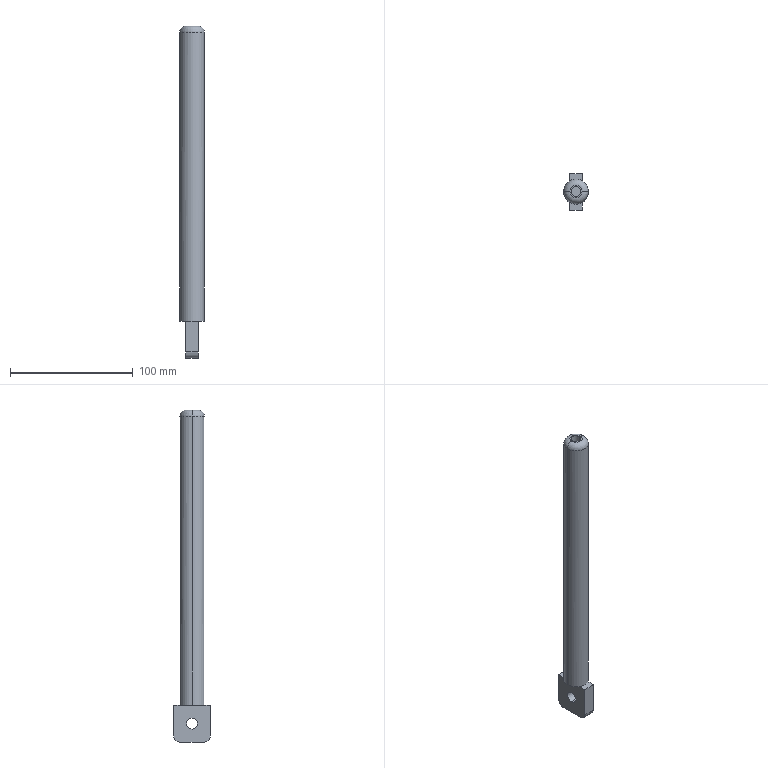Part | SolidWorks | features ICE 3, Fillet 2, Extrusion 1 | 1 solid | 21 faces | box 20 x 30 x 270 mm | volume 82350 mm3 | plane 11 | cylinder 8 | torus 2 | commonest cylinder face diameters 8 x2 9 x2 10 x2 20 x2
STEP:
#1=CARTESIAN_POINT('',(-4.,0.,220.));
#2=VERTEX_POINT('',#1);
#3=CARTESIAN_POINT('',(4.,0.,220.));
#4=VERTEX_POINT('',#3);
#5=CARTESIAN_POINT('',(0.,0.,220.));
#6=DIRECTION('',(0.,0.,1.));
#7=DIRECTION('',(1.,0.,0.));
#8=AXIS2_PLACEMENT_3D('',#5,#6,#7);
#9=CIRCLE('',#8,4.);
#10=EDGE_CURVE('',#2,#4,#9,.T.);
#11=ORIENTED_EDGE('',*,*,#10,.F.);
#12=CARTESIAN_POINT('',(-4.,0.,240.));
#13=VERTEX_POINT('',#12);
#14=CARTESIAN_POINT('',(-4.,0.,220.));
#15=DIRECTION('',(0.,0.,1.));
#16=VECTOR('',#15,1000.);
#17=LINE('',#14,#16);
#18=EDGE_CURVE('',#2,#13,#17,.T.);
#19=ORIENTED_EDGE('',*,*,#18,.T.);
#20=CARTESIAN_POINT('',(4.,0.,240.));
#21=VERTEX_POINT('',#20);
#22=CARTESIAN_POINT('',(0.,0.,240.));
#23=DIRECTION('',(0.,0.,1.));
#24=DIRECTION('',(1.,0.,0.));
#25=AXIS2_PLACEMENT_3D('',#22,#23,#24);
#26=CIRCLE('',#25,4.);
#27=EDGE_CURVE('',#13,#21,#26,.T.);
#28=ORIENTED_EDGE('',*,*,#27,.T.);
#29=CARTESIAN_POINT('',(4.,0.,220.));
#30=DIRECTION('',(0.,0.,1.));
#31=VECTOR('',#30,1000.);
#32=LINE('',#29,#31);
#33=EDGE_CURVE('',#4,#21,#32,.T.);
#34=ORIENTED_EDGE('',*,*,#33,.F.);
#35=EDGE_LOOP('',(#11,#19,#28,#34));
#36=FACE_OUTER_BOUND('',#35,.T.);
#37=CARTESIAN_POINT('',(0.,0.,220.));
#38=DIRECTION('',(0.,0.,1.));
#39=DIRECTION('',(1.,0.,0.));
#40=AXIS2_PLACEMENT_3D('',#37,#38,#39);
#41=CYLINDRICAL_SURFACE('',#40,4.);
#42=ADVANCED_FACE('',(#36),#41,.F.);
#43=CARTESIAN_POINT('',(-10.,0.,235.));
#44=VERTEX_POINT('',#43);
#45=CARTESIAN_POINT('',(10.,0.,235.));
#46=VERTEX_POINT('',#45);
#47=CARTESIAN_POINT('',(0.,0.,235.));
#48=DIRECTION('',(0.,0.,-1.));
#49=DIRECTION('',(1.,0.,0.));
#50=AXIS2_PLACEMENT_3D('',#47,#48,#49);
#51=CIRCLE('',#50,10.);
#52=EDGE_CURVE('',#44,#46,#51,.T.);
#53=ORIENTED_EDGE('',*,*,#52,.F.);
#54=CARTESIAN_POINT('',(-5.,0.,240.));
#55=VERTEX_POINT('',#54);
#56=CARTESIAN_POINT('',(-5.,0.,235.));
#57=DIRECTION('',(0.,1.,0.));
#58=DIRECTION('',(-1.,0.,0.));
#59=AXIS2_PLACEMENT_3D('',#56,#57,#58);
#60=CIRCLE('',#59,5.);
#61=EDGE_CURVE('',#44,#55,#60,.T.);
#62=ORIENTED_EDGE('',*,*,#61,.T.);
#63=CARTESIAN_POINT('',(5.,0.,240.));
#64=VERTEX_POINT('',#63);
#65=CARTESIAN_POINT('',(0.,0.,240.));
#66=DIRECTION('',(0.,0.,1.));
#67=DIRECTION('',(1.,0.,0.));
#68=AXIS2_PLACEMENT_3D('',#65,#66,#67);
#69=CIRCLE('',#68,5.);
#70=EDGE_CURVE('',#64,#55,#69,.T.);
#71=ORIENTED_EDGE('',*,*,#70,.F.);
#72=CARTESIAN_POINT('',(5.,0.,235.));
#73=DIRECTION('',(0.,-1.,0.));
#74=DIRECTION('',(0.,0.,-1.));
#75=AXIS2_PLACEMENT_3D('',#72,#73,#74);
#76=CIRCLE('',#75,5.);
#77=EDGE_CURVE('',#46,#64,#76,.T.);
#78=ORIENTED_EDGE('',*,*,#77,.F.);
#79=EDGE_LOOP('',(#53,#62,#71,#78));
#80=FACE_OUTER_BOUND('',#79,.T.);
#81=CARTESIAN_POINT('',(0.,0.,235.));
#82=DIRECTION('',(0.,0.,1.));
#83=DIRECTION('',(1.,0.,0.));
#84=AXIS2_PLACEMENT_3D('',#81,#82,#83);
#85=TOROIDAL_SURFACE('',#84,5.,5.);
#86=ADVANCED_FACE('',(#80),#85,.T.);
#87=CARTESIAN_POINT('',(-5.,0.,-19.5));
#88=VERTEX_POINT('',#87);
#89=CARTESIAN_POINT('',(-5.,0.,-10.5));
#90=VERTEX_POINT('',#89);
#91=CARTESIAN_POINT('',(-5.,0.,-15.));
#92=DIRECTION('',(-1.,0.,0.));
#93=DIRECTION('',(0.,0.,1.));
#94=AXIS2_PLACEMENT_3D('',#91,#92,#93);
#95=CIRCLE('',#94,4.5);
#96=EDGE_CURVE('',#88,#90,#95,.T.);
#97=ORIENTED_EDGE('',*,*,#96,.T.);
#98=CARTESIAN_POINT('',(5.,0.,-10.5));
#99=VERTEX_POINT('',#98);
#100=CARTESIAN_POINT('',(-33.,0.,-10.5));
#101=DIRECTION('',(1.,0.,0.));
#102=VECTOR('',#101,1000.);
#103=LINE('',#100,#102);
#104=EDGE_CURVE('',#90,#99,#103,.T.);
#105=ORIENTED_EDGE('',*,*,#104,.T.);
#106=CARTESIAN_POINT('',(5.,0.,-19.5));
#107=VERTEX_POINT('',#106);
#108=CARTESIAN_POINT('',(5.,0.,-15.));
#109=DIRECTION('',(1.,0.,0.));
#110=DIRECTION('',(0.,0.,-1.));
#111=AXIS2_PLACEMENT_3D('',#108,#109,#110);
#112=CIRCLE('',#111,4.5);
#113=EDGE_CURVE('',#99,#107,#112,.T.);
#114=ORIENTED_EDGE('',*,*,#113,.T.);
#115=CARTESIAN_POINT('',(-33.,0.,-19.5));
#116=DIRECTION('',(1.,0.,0.));
#117=VECTOR('',#116,1000.);
#118=LINE('',#115,#117);
#119=EDGE_CURVE('',#88,#107,#118,.T.);
#120=ORIENTED_EDGE('',*,*,#119,.F.);
#121=EDGE_LOOP('',(#97,#105,#114,#120));
#122=FACE_OUTER_BOUND('',#121,.T.);
#123=CARTESIAN_POINT('',(-33.,0.,-15.));
#124=DIRECTION('',(1.,0.,0.));
#125=DIRECTION('',(0.,0.,-1.));
#126=AXIS2_PLACEMENT_3D('',#123,#124,#125);
#127=CYLINDRICAL_SURFACE('',#126,4.5);
#128=ADVANCED_FACE('',(#122),#127,.F.);
#129=ORIENTED_EDGE('',*,*,#52,.T.);
#130=CARTESIAN_POINT('',(10.,0.,0.));
#131=VERTEX_POINT('',#130);
#132=CARTESIAN_POINT('',(10.,0.,240.));
#133=DIRECTION('',(0.,0.,-1.));
#134=VECTOR('',#133,1000.);
#135=LINE('',#132,#134);
#136=EDGE_CURVE('',#46,#131,#135,.T.);
#137=ORIENTED_EDGE('',*,*,#136,.T.);
#138=CARTESIAN_POINT('',(5.,8.66,0.));
#139=VERTEX_POINT('',#138);
#140=CARTESIAN_POINT('',(0.,0.,0.));
#141=DIRECTION('',(0.,0.,1.));
#142=DIRECTION('',(1.,0.,0.));
#143=AXIS2_PLACEMENT_3D('',#140,#141,#142);
#144=CIRCLE('',#143,10.);
#145=EDGE_CURVE('',#131,#139,#144,.T.);
#146=ORIENTED_EDGE('',*,*,#145,.T.);
#147=CARTESIAN_POINT('',(-5.,8.66,0.));
#148=VERTEX_POINT('',#147);
#149=CARTESIAN_POINT('',(0.,0.,0.));
#150=DIRECTION('',(0.,0.,1.));
#151=DIRECTION('',(1.,0.,0.));
#152=AXIS2_PLACEMENT_3D('',#149,#150,#151);
#153=CIRCLE('',#152,10.);
#154=EDGE_CURVE('',#139,#148,#153,.T.);
#155=ORIENTED_EDGE('',*,*,#154,.T.);
#156=CARTESIAN_POINT('',(-10.,0.,0.));
#157=VERTEX_POINT('',#156);
#158=CARTESIAN_POINT('',(0.,0.,0.));
#159=DIRECTION('',(0.,0.,1.));
#160=DIRECTION('',(1.,0.,0.));
#161=AXIS2_PLACEMENT_3D('',#158,#159,#160);
#162=CIRCLE('',#161,10.);
#163=EDGE_CURVE('',#148,#157,#162,.T.);
#164=ORIENTED_EDGE('',*,*,#163,.T.);
#165=CARTESIAN_POINT('',(-10.,0.,240.));
#166=DIRECTION('',(0.,0.,-1.));
#167=VECTOR('',#166,1000.);
#168=LINE('',#165,#167);
#169=EDGE_CURVE('',#44,#157,#168,.T.);
#170=ORIENTED_EDGE('',*,*,#169,.F.);
#171=EDGE_LOOP('',(#129,#137,#146,#155,#164,#170));
#172=FACE_OUTER_BOUND('',#171,.T.);
#173=CARTESIAN_POINT('',(0.,0.,240.));
#174=DIRECTION('',(0.,0.,-1.));
#175=DIRECTION('',(-1.,0.,0.));
#176=AXIS2_PLACEMENT_3D('',#173,#174,#175);
#177=CYLINDRICAL_SURFACE('',#176,10.);
#178=ADVANCED_FACE('',(#172),#177,.T.);
#179=CARTESIAN_POINT('',(5.,-8.66,0.));
#180=VERTEX_POINT('',#179);
#181=CARTESIAN_POINT('',(5.,-15.,0.));
#182=DIRECTION('',(0.,-1.,0.));
#183=VECTOR('',#182,1000.);
#184=LINE('',#181,#183);
#185=EDGE_CURVE('',#139,#180,#184,.T.);
#186=ORIENTED_EDGE('',*,*,#185,.F.);
#187=ORIENTED_EDGE('',*,*,#145,.F.);
#188=CARTESIAN_POINT('',(0.,0.,0.));
#189=DIRECTION('',(0.,0.,1.));
#190=DIRECTION('',(1.,0.,0.));
#191=AXIS2_PLACEMENT_3D('',#188,#189,#190);
#192=CIRCLE('',#191,10.);
#193=EDGE_CURVE('',#180,#131,#192,.T.);
#194=ORIENTED_EDGE('',*,*,#193,.F.);
#195=EDGE_LOOP('',(#186,#187,#194));
#196=FACE_OUTER_BOUND('',#195,.T.);
#197=CARTESIAN_POINT('',(0.,0.,0.));
#198=DIRECTION('',(0.,0.,1.));
#199=DIRECTION('',(1.,0.,0.));
#200=AXIS2_PLACEMENT_3D('',#197,#198,#199);
#201=PLANE('',#200);
#202=ADVANCED_FACE('',(#196),#201,.F.);
#203=ORIENTED_EDGE('',*,*,#136,.F.);
#204=CARTESIAN_POINT('',(0.,0.,235.));
#205=DIRECTION('',(0.,0.,-1.));
#206=DIRECTION('',(1.,0.,0.));
#207=AXIS2_PLACEMENT_3D('',#204,#205,#206);
#208=CIRCLE('',#207,10.);
#209=EDGE_CURVE('',#46,#44,#208,.T.);
#210=ORIENTED_EDGE('',*,*,#209,.T.);
#211=ORIENTED_EDGE('',*,*,#169,.T.);
#212=CARTESIAN_POINT('',(-5.,-8.66,0.));
#213=VERTEX_POINT('',#212);
#214=CARTESIAN_POINT('',(0.,0.,0.));
#215=DIRECTION('',(0.,0.,1.));
#216=DIRECTION('',(1.,0.,0.));
#217=AXIS2_PLACEMENT_3D('',#214,#215,#216);
#218=CIRCLE('',#217,10.);
#219=EDGE_CURVE('',#157,#213,#218,.T.);
#220=ORIENTED_EDGE('',*,*,#219,.T.);
#221=CARTESIAN_POINT('',(0.,0.,0.));
#222=DIRECTION('',(0.,0.,1.));
#223=DIRECTION('',(1.,0.,0.));
#224=AXIS2_PLACEMENT_3D('',#221,#222,#223);
#225=CIRCLE('',#224,10.);
#226=EDGE_CURVE('',#213,#180,#225,.T.);
#227=ORIENTED_EDGE('',*,*,#226,.T.);
#228=ORIENTED_EDGE('',*,*,#193,.T.);
#229=EDGE_LOOP('',(#203,#210,#211,#220,#227,#228));
#230=FACE_OUTER_BOUND('',#229,.T.);
#231=CARTESIAN_POINT('',(0.,0.,240.));
#232=DIRECTION('',(0.,0.,-1.));
#233=DIRECTION('',(-1.,0.,0.));
#234=AXIS2_PLACEMENT_3D('',#231,#232,#233);
#235=CYLINDRICAL_SURFACE('',#234,10.);
#236=ADVANCED_FACE('',(#230),#235,.T.);
#237=CARTESIAN_POINT('',(0.,0.,240.));
#238=DIRECTION('',(0.,0.,1.));
#239=DIRECTION('',(1.,0.,0.));
#240=AXIS2_PLACEMENT_3D('',#237,#238,#239);
#241=CIRCLE('',#240,4.);
#242=EDGE_CURVE('',#21,#13,#241,.T.);
#243=ORIENTED_EDGE('',*,*,#242,.F.);
#244=ORIENTED_EDGE('',*,*,#27,.F.);
#245=EDGE_LOOP('',(#243,#244));
#246=FACE_BOUND('',#245,.T.);
#247=ORIENTED_EDGE('',*,*,#70,.T.);
#248=CARTESIAN_POINT('',(0.,0.,240.));
#249=DIRECTION('',(0.,0.,1.));
#250=DIRECTION('',(1.,0.,0.));
#251=AXIS2_PLACEMENT_3D('',#248,#249,#250);
#252=CIRCLE('',#251,5.);
#253=EDGE_CURVE('',#55,#64,#252,.T.);
#254=ORIENTED_EDGE('',*,*,#253,.T.);
#255=EDGE_LOOP('',(#247,#254));
#256=FACE_OUTER_BOUND('',#255,.T.);
#257=CARTESIAN_POINT('',(0.,0.,240.));
#258=DIRECTION('',(0.,0.,1.));
#259=DIRECTION('',(1.,0.,0.));
#260=AXIS2_PLACEMENT_3D('',#257,#258,#259);
#261=PLANE('',#260);
#262=ADVANCED_FACE('',(#246,#256),#261,.T.);
#263=ORIENTED_EDGE('',*,*,#163,.F.);
#264=CARTESIAN_POINT('',(-5.,-15.,0.));
#265=DIRECTION('',(0.,-1.,0.));
#266=VECTOR('',#265,1000.);
#267=LINE('',#264,#266);
#268=EDGE_CURVE('',#148,#213,#267,.T.);
#269=ORIENTED_EDGE('',*,*,#268,.T.);
#270=ORIENTED_EDGE('',*,*,#219,.F.);
#271=EDGE_LOOP('',(#263,#269,#270));
#272=FACE_OUTER_BOUND('',#271,.T.);
#273=CARTESIAN_POINT('',(0.,0.,0.));
#274=DIRECTION('',(0.,0.,1.));
#275=DIRECTION('',(1.,0.,0.));
#276=AXIS2_PLACEMENT_3D('',#273,#274,#275);
#277=PLANE('',#276);
#278=ADVANCED_FACE('',(#272),#277,.F.);
#279=ORIENTED_EDGE('',*,*,#154,.F.);
#280=CARTESIAN_POINT('',(5.,15.,0.));
#281=VERTEX_POINT('',#280);
#282=CARTESIAN_POINT('',(5.,-15.,0.));
#283=DIRECTION('',(0.,-1.,0.));
#284=VECTOR('',#283,1000.);
#285=LINE('',#282,#284);
#286=EDGE_CURVE('',#281,#139,#285,.T.);
#287=ORIENTED_EDGE('',*,*,#286,.F.);
#288=CARTESIAN_POINT('',(-5.,15.,0.));
#289=VERTEX_POINT('',#288);
#290=CARTESIAN_POINT('',(5.,15.,0.));
#291=DIRECTION('',(-1.,0.,0.));
#292=VECTOR('',#291,1000.);
#293=LINE('',#290,#292);
#294=EDGE_CURVE('',#281,#289,#293,.T.);
#295=ORIENTED_EDGE('',*,*,#294,.T.);
#296=CARTESIAN_POINT('',(-5.,-15.,0.));
#297=DIRECTION('',(0.,-1.,0.));
#298=VECTOR('',#297,1000.);
#299=LINE('',#296,#298);
#300=EDGE_CURVE('',#289,#148,#299,.T.);
#301=ORIENTED_EDGE('',*,*,#300,.T.);
#302=EDGE_LOOP('',(#279,#287,#295,#301));
#303=FACE_OUTER_BOUND('',#302,.T.);
#304=CARTESIAN_POINT('',(5.,-15.,0.));
#305=DIRECTION('',(0.,0.,-1.));
#306=DIRECTION('',(-1.,0.,0.));
#307=AXIS2_PLACEMENT_3D('',#304,#305,#306);
#308=PLANE('',#307);
#309=ADVANCED_FACE('',(#303),#308,.F.);
#310=CARTESIAN_POINT('',(-5.,-10.,-30.));
#311=VERTEX_POINT('',#310);
#312=CARTESIAN_POINT('',(-5.,10.,-30.));
#313=VERTEX_POINT('',#312);
#314=CARTESIAN_POINT('',(-5.,-15.,-30.));
#315=DIRECTION('',(0.,1.,0.));
#316=VECTOR('',#315,1000.);
#317=LINE('',#314,#316);
#318=EDGE_CURVE('',#311,#313,#317,.T.);
#319=ORIENTED_EDGE('',*,*,#318,.T.);
#320=CARTESIAN_POINT('',(5.,10.,-30.));
#321=VERTEX_POINT('',#320);
#322=CARTESIAN_POINT('',(5.,10.,-30.));
#323=DIRECTION('',(1.,0.,0.));
#324=VECTOR('',#323,1000.);
#325=LINE('',#322,#324);
#326=EDGE_CURVE('',#313,#321,#325,.T.);
#327=ORIENTED_EDGE('',*,*,#326,.T.);
#328=CARTESIAN_POINT('',(5.,-10.,-30.));
#329=VERTEX_POINT('',#328);
#330=CARTESIAN_POINT('',(5.,-15.,-30.));
#331=DIRECTION('',(0.,1.,0.));
#332=VECTOR('',#331,1000.);
#333=LINE('',#330,#332);
#334=EDGE_CURVE('',#329,#321,#333,.T.);
#335=ORIENTED_EDGE('',*,*,#334,.F.);
#336=CARTESIAN_POINT('',(5.,-10.,-30.));
#337=DIRECTION('',(-1.,0.,0.));
#338=VECTOR('',#337,1000.);
#339=LINE('',#336,#338);
#340=EDGE_CURVE('',#329,#311,#339,.T.);
#341=ORIENTED_EDGE('',*,*,#340,.T.);
#342=EDGE_LOOP('',(#319,#327,#335,#341));
#343=FACE_OUTER_BOUND('',#342,.T.);
#344=CARTESIAN_POINT('',(5.,-15.,-30.));
#345=DIRECTION('',(0.,0.,1.));
#346=DIRECTION('',(1.,0.,0.));
#347=AXIS2_PLACEMENT_3D('',#344,#345,#346);
#348=PLANE('',#347);
#349=ADVANCED_FACE('',(#343),#348,.F.);
#350=CARTESIAN_POINT('',(5.,15.,-25.));
#351=VERTEX_POINT('',#350);
#352=CARTESIAN_POINT('',(5.,15.,0.));
#353=DIRECTION('',(0.,0.,1.));
#354=VECTOR('',#353,1000.);
#355=LINE('',#352,#354);
#356=EDGE_CURVE('',#351,#281,#355,.T.);
#357=ORIENTED_EDGE('',*,*,#356,.F.);
#358=CARTESIAN_POINT('',(-5.,15.,-25.));
#359=VERTEX_POINT('',#358);
#360=CARTESIAN_POINT('',(5.,15.,-25.));
#361=DIRECTION('',(-1.,0.,0.));
#362=VECTOR('',#361,1000.);
#363=LINE('',#360,#362);
#364=EDGE_CURVE('',#351,#359,#363,.T.);
#365=ORIENTED_EDGE('',*,*,#364,.T.);
#366=CARTESIAN_POINT('',(-5.,15.,0.));
#367=DIRECTION('',(0.,0.,1.));
#368=VECTOR('',#367,1000.);
#369=LINE('',#366,#368);
#370=EDGE_CURVE('',#359,#289,#369,.T.);
#371=ORIENTED_EDGE('',*,*,#370,.T.);
#372=ORIENTED_EDGE('',*,*,#294,.F.);
#373=EDGE_LOOP('',(#357,#365,#371,#372));
#374=FACE_OUTER_BOUND('',#373,.T.);
#375=CARTESIAN_POINT('',(5.,15.,0.));
#376=DIRECTION('',(0.,-1.,0.));
#377=DIRECTION('',(0.,0.,-1.));
#378=AXIS2_PLACEMENT_3D('',#375,#376,#377);
#379=PLANE('',#378);
#380=ADVANCED_FACE('',(#374),#379,.F.);
#381=ORIENTED_EDGE('',*,*,#226,.F.);
#382=CARTESIAN_POINT('',(-5.,-15.,0.));
#383=VERTEX_POINT('',#382);
#384=CARTESIAN_POINT('',(-5.,-15.,0.));
#385=DIRECTION('',(0.,-1.,0.));
#386=VECTOR('',#385,1000.);
#387=LINE('',#384,#386);
#388=EDGE_CURVE('',#213,#383,#387,.T.);
#389=ORIENTED_EDGE('',*,*,#388,.T.);
#390=CARTESIAN_POINT('',(5.,-15.,0.));
#391=VERTEX_POINT('',#390);
#392=CARTESIAN_POINT('',(5.,-15.,0.));
#393=DIRECTION('',(-1.,0.,0.));
#394=VECTOR('',#393,1000.);
#395=LINE('',#392,#394);
#396=EDGE_CURVE('',#391,#383,#395,.T.);
#397=ORIENTED_EDGE('',*,*,#396,.F.);
#398=CARTESIAN_POINT('',(5.,-15.,0.));
#399=DIRECTION('',(0.,-1.,0.));
#400=VECTOR('',#399,1000.);
#401=LINE('',#398,#400);
#402=EDGE_CURVE('',#180,#391,#401,.T.);
#403=ORIENTED_EDGE('',*,*,#402,.F.);
#404=EDGE_LOOP('',(#381,#389,#397,#403));
#405=FACE_OUTER_BOUND('',#404,.T.);
#406=CARTESIAN_POINT('',(5.,-15.,0.));
#407=DIRECTION('',(0.,0.,-1.));
#408=DIRECTION('',(-1.,0.,0.));
#409=AXIS2_PLACEMENT_3D('',#406,#407,#408);
#410=PLANE('',#409);
#411=ADVANCED_FACE('',(#405),#410,.F.);
#412=CARTESIAN_POINT('',(-5.,-15.,-25.));
#413=VERTEX_POINT('',#412);
#414=CARTESIAN_POINT('',(-5.,-15.,0.));
#415=DIRECTION('',(0.,0.,-1.));
#416=VECTOR('',#415,1000.);
#417=LINE('',#414,#416);
#418=EDGE_CURVE('',#383,#413,#417,.T.);
#419=ORIENTED_EDGE('',*,*,#418,.T.);
#420=CARTESIAN_POINT('',(5.,-15.,-25.));
#421=VERTEX_POINT('',#420);
#422=CARTESIAN_POINT('',(5.,-15.,-25.));
#423=DIRECTION('',(1.,0.,0.));
#424=VECTOR('',#423,1000.);
#425=LINE('',#422,#424);
#426=EDGE_CURVE('',#413,#421,#425,.T.);
#427=ORIENTED_EDGE('',*,*,#426,.T.);
#428=CARTESIAN_POINT('',(5.,-15.,0.));
#429=DIRECTION('',(0.,0.,-1.));
#430=VECTOR('',#429,1000.);
#431=LINE('',#428,#430);
#432=EDGE_CURVE('',#391,#421,#431,.T.);
#433=ORIENTED_EDGE('',*,*,#432,.F.);
#434=ORIENTED_EDGE('',*,*,#396,.T.);
#435=EDGE_LOOP('',(#419,#427,#433,#434));
#436=FACE_OUTER_BOUND('',#435,.T.);
#437=CARTESIAN_POINT('',(5.,-15.,0.));
#438=DIRECTION('',(0.,1.,0.));
#439=DIRECTION('',(0.,0.,1.));
#440=AXIS2_PLACEMENT_3D('',#437,#438,#439);
#441=PLANE('',#440);
#442=ADVANCED_FACE('',(#436),#441,.F.);
#443=CARTESIAN_POINT('',(5.,0.,-15.));
#444=DIRECTION('',(1.,0.,0.));
#445=DIRECTION('',(0.,0.,-1.));
#446=AXIS2_PLACEMENT_3D('',#443,#444,#445);
#447=CIRCLE('',#446,4.5);
#448=EDGE_CURVE('',#107,#99,#447,.T.);
#449=ORIENTED_EDGE('',*,*,#448,.F.);
#450=ORIENTED_EDGE('',*,*,#113,.F.);
#451=EDGE_LOOP('',(#449,#450));
#452=FACE_BOUND('',#451,.T.);
#453=ORIENTED_EDGE('',*,*,#334,.T.);
#454=CARTESIAN_POINT('',(5.,10.,-25.));
#455=DIRECTION('',(1.,0.,0.));
#456=DIRECTION('',(0.,0.,1.));
#457=AXIS2_PLACEMENT_3D('',#454,#455,#456);
#458=CIRCLE('',#457,5.);
#459=EDGE_CURVE('',#321,#351,#458,.T.);
#460=ORIENTED_EDGE('',*,*,#459,.T.);
#461=ORIENTED_EDGE('',*,*,#356,.T.);
#462=ORIENTED_EDGE('',*,*,#286,.T.);
#463=ORIENTED_EDGE('',*,*,#185,.T.);
#464=ORIENTED_EDGE('',*,*,#402,.T.);
#465=ORIENTED_EDGE('',*,*,#432,.T.);
#466=CARTESIAN_POINT('',(5.,-10.,-25.));
#467=DIRECTION('',(1.,0.,0.));
#468=DIRECTION('',(0.,0.,1.));
#469=AXIS2_PLACEMENT_3D('',#466,#467,#468);
#470=CIRCLE('',#469,5.);
#471=EDGE_CURVE('',#421,#329,#470,.T.);
#472=ORIENTED_EDGE('',*,*,#471,.T.);
#473=EDGE_LOOP('',(#453,#460,#461,#462,#463,#464,#465,#472));
#474=FACE_OUTER_BOUND('',#473,.T.);
#475=CARTESIAN_POINT('',(5.,0.,0.));
#476=DIRECTION('',(-1.,0.,0.));
#477=DIRECTION('',(0.,0.,1.));
#478=AXIS2_PLACEMENT_3D('',#475,#476,#477);
#479=PLANE('',#478);
#480=ADVANCED_FACE('',(#452,#474),#479,.F.);
#481=ORIENTED_EDGE('',*,*,#96,.F.);
#482=CARTESIAN_POINT('',(-5.,0.,-15.));
#483=DIRECTION('',(-1.,0.,0.));
#484=DIRECTION('',(0.,0.,1.));
#485=AXIS2_PLACEMENT_3D('',#482,#483,#484);
#486=CIRCLE('',#485,4.5);
#487=EDGE_CURVE('',#90,#88,#486,.T.);
#488=ORIENTED_EDGE('',*,*,#487,.F.);
#489=EDGE_LOOP('',(#481,#488));
#490=FACE_BOUND('',#489,.T.);
#491=ORIENTED_EDGE('',*,*,#370,.F.);
#492=CARTESIAN_POINT('',(-5.,10.,-25.));
#493=DIRECTION('',(-1.,0.,0.));
#494=DIRECTION('',(0.,0.,1.));
#495=AXIS2_PLACEMENT_3D('',#492,#493,#494);
#496=CIRCLE('',#495,5.);
#497=EDGE_CURVE('',#359,#313,#496,.T.);
#498=ORIENTED_EDGE('',*,*,#497,.T.);
#499=ORIENTED_EDGE('',*,*,#318,.F.);
#500=CARTESIAN_POINT('',(-5.,-10.,-25.));
#501=DIRECTION('',(-1.,0.,0.));
#502=DIRECTION('',(0.,0.,1.));
#503=AXIS2_PLACEMENT_3D('',#500,#501,#502);
#504=CIRCLE('',#503,5.);
#505=EDGE_CURVE('',#311,#413,#504,.T.);
#506=ORIENTED_EDGE('',*,*,#505,.T.);
#507=ORIENTED_EDGE('',*,*,#418,.F.);
#508=ORIENTED_EDGE('',*,*,#388,.F.);
#509=ORIENTED_EDGE('',*,*,#268,.F.);
#510=ORIENTED_EDGE('',*,*,#300,.F.);
#511=EDGE_LOOP('',(#491,#498,#499,#506,#507,#508,#509,#510));
#512=FACE_OUTER_BOUND('',#511,.T.);
#513=CARTESIAN_POINT('',(-5.,0.,0.));
#514=DIRECTION('',(-1.,0.,0.));
#515=DIRECTION('',(0.,0.,1.));
#516=AXIS2_PLACEMENT_3D('',#513,#514,#515);
#517=PLANE('',#516);
#518=ADVANCED_FACE('',(#490,#512),#517,.T.);
#519=ORIENTED_EDGE('',*,*,#104,.F.);
#520=ORIENTED_EDGE('',*,*,#487,.T.);
#521=ORIENTED_EDGE('',*,*,#119,.T.);
#522=ORIENTED_EDGE('',*,*,#448,.T.);
#523=EDGE_LOOP('',(#519,#520,#521,#522));
#524=FACE_OUTER_BOUND('',#523,.T.);
#525=CARTESIAN_POINT('',(-33.,0.,-15.));
#526=DIRECTION('',(1.,0.,0.));
#527=DIRECTION('',(0.,0.,-1.));
#528=AXIS2_PLACEMENT_3D('',#525,#526,#527);
#529=CYLINDRICAL_SURFACE('',#528,4.5);
#530=ADVANCED_FACE('',(#524),#529,.F.);
#531=ORIENTED_EDGE('',*,*,#459,.F.);
#532=ORIENTED_EDGE('',*,*,#326,.F.);
#533=ORIENTED_EDGE('',*,*,#497,.F.);
#534=ORIENTED_EDGE('',*,*,#364,.F.);
#535=EDGE_LOOP('',(#531,#532,#533,#534));
#536=FACE_OUTER_BOUND('',#535,.T.);
#537=CARTESIAN_POINT('',(5.,10.,-25.));
#538=DIRECTION('',(-1.,0.,0.));
#539=DIRECTION('',(0.,0.,1.));
#540=AXIS2_PLACEMENT_3D('',#537,#538,#539);
#541=CYLINDRICAL_SURFACE('',#540,5.);
#542=ADVANCED_FACE('',(#536),#541,.T.);
#543=ORIENTED_EDGE('',*,*,#471,.F.);
#544=ORIENTED_EDGE('',*,*,#426,.F.);
#545=ORIENTED_EDGE('',*,*,#505,.F.);
#546=ORIENTED_EDGE('',*,*,#340,.F.);
#547=EDGE_LOOP('',(#543,#544,#545,#546));
#548=FACE_OUTER_BOUND('',#547,.T.);
#549=CARTESIAN_POINT('',(5.,-10.,-25.));
#550=DIRECTION('',(-1.,0.,0.));
#551=DIRECTION('',(0.,0.,1.));
#552=AXIS2_PLACEMENT_3D('',#549,#550,#551);
#553=CYLINDRICAL_SURFACE('',#552,5.);
#554=ADVANCED_FACE('',(#548),#553,.T.);
#555=ORIENTED_EDGE('',*,*,#61,.F.);
#556=ORIENTED_EDGE('',*,*,#209,.F.);
#557=ORIENTED_EDGE('',*,*,#77,.T.);
#558=ORIENTED_EDGE('',*,*,#253,.F.);
#559=EDGE_LOOP('',(#555,#556,#557,#558));
#560=FACE_OUTER_BOUND('',#559,.T.);
#561=CARTESIAN_POINT('',(0.,0.,235.));
#562=DIRECTION('',(0.,0.,1.));
#563=DIRECTION('',(1.,0.,0.));
#564=AXIS2_PLACEMENT_3D('',#561,#562,#563);
#565=TOROIDAL_SURFACE('',#564,5.,5.);
#566=ADVANCED_FACE('',(#560),#565,.T.);
#567=ORIENTED_EDGE('',*,*,#18,.F.);
#568=CARTESIAN_POINT('',(0.,0.,220.));
#569=DIRECTION('',(0.,0.,1.));
#570=DIRECTION('',(1.,0.,0.));
#571=AXIS2_PLACEMENT_3D('',#568,#569,#570);
#572=CIRCLE('',#571,4.);
#573=EDGE_CURVE('',#4,#2,#572,.T.);
#574=ORIENTED_EDGE('',*,*,#573,.F.);
#575=ORIENTED_EDGE('',*,*,#33,.T.);
#576=ORIENTED_EDGE('',*,*,#242,.T.);
#577=EDGE_LOOP('',(#567,#574,#575,#576));
#578=FACE_OUTER_BOUND('',#577,.T.);
#579=CARTESIAN_POINT('',(0.,0.,220.));
#580=DIRECTION('',(0.,0.,1.));
#581=DIRECTION('',(1.,0.,0.));
#582=AXIS2_PLACEMENT_3D('',#579,#580,#581);
#583=CYLINDRICAL_SURFACE('',#582,4.);
#584=ADVANCED_FACE('',(#578),#583,.F.);
#585=ORIENTED_EDGE('',*,*,#573,.T.);
#586=ORIENTED_EDGE('',*,*,#10,.T.);
#587=EDGE_LOOP('',(#585,#586));
#588=FACE_OUTER_BOUND('',#587,.T.);
#589=CARTESIAN_POINT('',(0.,0.,220.));
#590=DIRECTION('',(0.,0.,1.));
#591=DIRECTION('',(1.,0.,0.));
#592=AXIS2_PLACEMENT_3D('',#589,#590,#591);
#593=PLANE('',#592);
#594=ADVANCED_FACE('',(#588),#593,.T.);
#595=CLOSED_SHELL('',(#42,#86,#128,#178,#202,#236,#262,#278,#309,#349,#380,#411,#442,#480,#518,#530,#542,#554,#566,#584,#594));
#596=MANIFOLD_SOLID_BREP('',#595);
#597=CARTESIAN_POINT('',(0.,0.,0.));
#598=DIRECTION('',(0.,0.,1.));
#599=DIRECTION('',(1.,0.,0.));
#600=AXIS2_PLACEMENT_3D('',#597,#598,#599);
#601=(LENGTH_UNIT()NAMED_UNIT(*)SI_UNIT(.MILLI.,.METRE.));
#602=UNCERTAINTY_MEASURE_WITH_UNIT(LENGTH_MEASURE(0.00001),#601,'','');
#603=(NAMED_UNIT(*)PLANE_ANGLE_UNIT()SI_UNIT($,.RADIAN.));
#604=(NAMED_UNIT(*)SI_UNIT($,.STERADIAN.)SOLID_ANGLE_UNIT());
#605=(GEOMETRIC_REPRESENTATION_CONTEXT(3)GLOBAL_UNCERTAINTY_ASSIGNED_CONTEXT((#602))GLOBAL_UNIT_ASSIGNED_CONTEXT((#601,#603,#604))REPRESENTATION_CONTEXT('',''));
#606=ADVANCED_BREP_SHAPE_REPRESENTATION('',(#596,#600),#605);